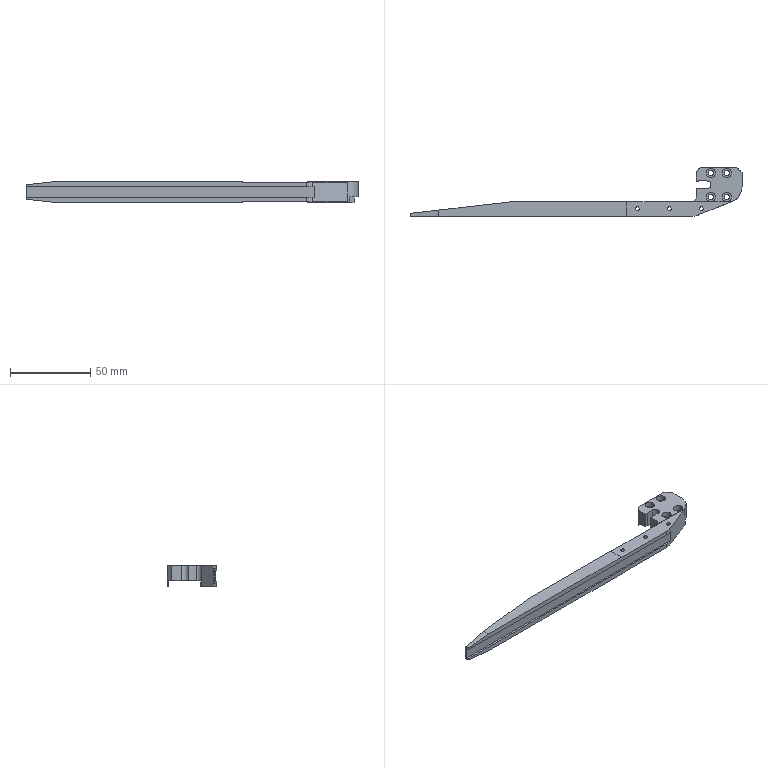CAM job | NX | 3+2 milling, drilling | part box 207.5 x 30.8 x 13 mm | stock box 212.5 x 35.8 x 15 mm
Tools:
number,name,description,diameter,corner_radius,flute_length,length,flutes
4,D4,平底铣刀-粗,4.0,0.0,25.0,75.0,2
6,D6,平底铣刀-粗,6.0,0.0,25.0,75.0,2
9,D10,平底铣刀-粗,10.0,0.0,35.0,75.0,2
17,D3-J,平底铣刀-精,3.0,0.0,50.0,75.0,2
11,D4-J,平底铣刀-精,4.0,0.0,50.0,75.0,2
7,D6-J,平底铣刀-精,6.0,0.0,25.0,75.0,2
1,D80R0.8飞刀,圆鼻刀-粗,80.0,0.8,50.0,75.0,2
2,D6倒角刀,倒角刀,6.0,0.0,3.0,25.0,2
18,R2,圆球刀,4.0,2.0,10.0,50.0,2
20,M3X0.5,丝锥,2.5,0.0,35.0,50.0,2
12,ZT2.5,钻头,2.5,0.0,35.0,50.0,2
13,ZT3.4,钻头,3.4,0.0,35.0,50.0,2
Operations:
program,operation,operation_type,tool,method,geometry_group,spindle_rpm,surface_speed,feed_per_tooth,feed_cut,feed_plunge,cut_length_mm,path_length_mm,cut_time_min,machine_time_min
C,底壁铣分层开粗-中_COPY_1,VolumeBased25DMillingOperation,D6,分层开粗-切深K-步距G,W-C,8000.0,150.796,0.125,2000.0,100.0,766.29,785.441,0.3831,0.3851
C,平面去毛刺6X45L_COPY_1,SurfaceContour,D6倒角刀,爬面_倒角-切深0-步距G,W-C,6500.0,122.519,0.1154,1500.0,100.0,355.731,465.09,0.2372,0.2481
C,底壁铣精光侧面-中-选底面_COPY_2,VolumeBased25DMillingOperation,D6-J,侧刃精光-切深K-步距G,W-C,8000.0,150.792,0.0625,1000.0,100.0,384.154,404.183,0.3842,0.3862
B,动态开粗D10_COPY,CavityMilling,D10,动态开粗-切深K-步距K,W-B,8000.0,251.32,0.25,4000.0,100.0,16838.72,16874.52,4.21,4.213
B,型腔铣开粗-中_COPY_1,CavityMilling,D10,分层开粗-切深K-步距G,W-B,8000.0,251.32,0.25,4000.0,100.0,354.561,475.898,0.0886,0.1058
B,底壁铣分层开粗-中_COPY,VolumeBased25DMillingOperation,D10,分层开粗-切深K-步距G,W-B,8000.0,251.32,0.25,4000.0,100.0,246.766,267.766,0.0617,0.0638
B,铣沉头_1,CylinderMilling,D4,METHOD,W-B,8000.0,100.531,0.075,1200.0,100.0,442.604,650.004,0.3688,0.3896
B,铣孔_1,CylinderMilling,D4-J,METHOD,W-B,8000.0,100.531,0.0375,600.0,100.0,35.391,257.591,0.059,0.0812
B,曲面D4R2_COPY,SurfaceContour,R2,METHOD,W-B,6000.0,75.0,0.2083,3500.0,100.0,792.492,826.514,0.2264,0.2298
B,钻倒角_2,Operation,D6倒角刀,METHOD,W-B,8000.0,150.796,0.0625,1000.0,0.0,14.25,115.547,0.0143,0.0244
B,平面去毛刺6X45L_COPY,SurfaceContour,D6倒角刀,爬面_倒角-切深0-步距G,W-B,6500.0,122.519,0.1154,1500.0,100.0,544.542,762.283,0.363,0.3848
B,底壁铣飞面精光_COPY,VolumeBased25DMillingOperation,D6-J,侧刃精光-切深K-步距G,W-B,8000.0,251.32,0.0625,1000.0,100.0,1151.285,1187.285,1.151,1.155
B,底壁铣精光底面-中_COPY,VolumeBased25DMillingOperation,D6-J,精光步距切深关,W-B,8000.0,150.792,0.0625,1000.0,100.0,207.051,228.251,0.2071,0.2092
B,底壁铣精光侧面-中-选底面_COPY_1,VolumeBased25DMillingOperation,D6-J,侧刃精光-切深K-步距G,W-B,8000.0,150.792,0.0625,1000.0,100.0,77.921,100.121,0.0779,0.0801
B,底壁铣精光侧面-中_COPY,VolumeBased25DMillingOperation,D6-J,侧刃精光-切深K-步距G,W-B,8000.0,150.792,0.0625,1000.0,100.0,21.386,42.586,0.0214,0.0235
A,顶面,FaceMilling,D80R0.8飞刀,侧刃精光-切深K-步距G,W-A,4000.0,1005.31,0.125,1000.0,100.0,301.5,337.5,0.3015,0.3051
A,打点-深0.8,Operation,D6倒角刀,NONE,W-A,8000.0,150.796,0.0312,500.0,90.0,12.6,155.885,0.0252,0.0395
A,通孔-M3螺纹底孔,Operation,ZT2.5,NONE,W-A,3000.0,23.562,0.05,300.0,90.0,58.353,198.756,0.1945,0.2086
A,通孔-3-4,Operation,ZT3.4,NONE,W-A,3000.0,32.044,0.02,120.0,90.0,54.486,187.105,0.454,0.4673
A,型腔铣开粗-中_COPY,CavityMilling,D10,分层开粗-切深K-步距G,W-A,8000.0,251.32,0.25,4000.0,100.0,46227.193,46968.293,11.557,11.67
A,底精_1,VolumeBased25DMillingOperation,D6-J,METHOD,W-A,6000.0,113.0,0.2083,1200.0,100.0,214.337,253.937,0.1786,0.1826
A,底精_2,VolumeBased25DMillingOperation,D6-J,METHOD,W-A,6000.0,113.0,0.2083,1200.0,100.0,162.473,208.273,0.1354,0.14
A,外形侧面,ZLevelMilling,D3-J,METHOD,W-A,9000.0,84.823,0.1111,2000.0,80.0,1224.776,1303.515,0.6126,0.6205
A,曲面D4R2,SurfaceContour,R2,METHOD,W-A,6000.0,75.0,0.2083,3500.0,100.0,781.932,815.953,0.2234,0.2268
A,仅选体,SurfaceContour,D6倒角刀,METHOD,W-A,8000.0,150.796,0.1875,3000.0,100.0,534.332,1214.59,0.1781,0.2461
A,钻倒角_1,Operation,D6倒角刀,METHOD,W-A,8000.0,150.796,0.0312,500.0,0.0,14.25,115.547,0.0285,0.0386
A,通孔-攻牙M3,Operation,M3X0.5,METHOD,W-A,800.0,6.283,0.0003,0.5,90.0,49.2,181.05,98.4,98.413
A,底侧精_3,VolumeBased25DMillingOperation,D6-J,METHOD,W-A,6000.0,113.0,0.1,1200.0,100.0,56.309,171.093,0.0469,0.0584
A,外形半精_2,VolumeBased25DMillingOperation,D6-J,METHOD,W-A,6000.0,113.097,0.0833,1000.0,100.0,477.33,542.33,0.4773,0.4838
A,底壁铣精光侧面-中-选底面_COPY,VolumeBased25DMillingOperation,D6-J,侧刃精光-切深K-步距G,W-A,6000.0,113.097,0.0667,800.0,100.0,79.356,115.912,0.0992,0.1029